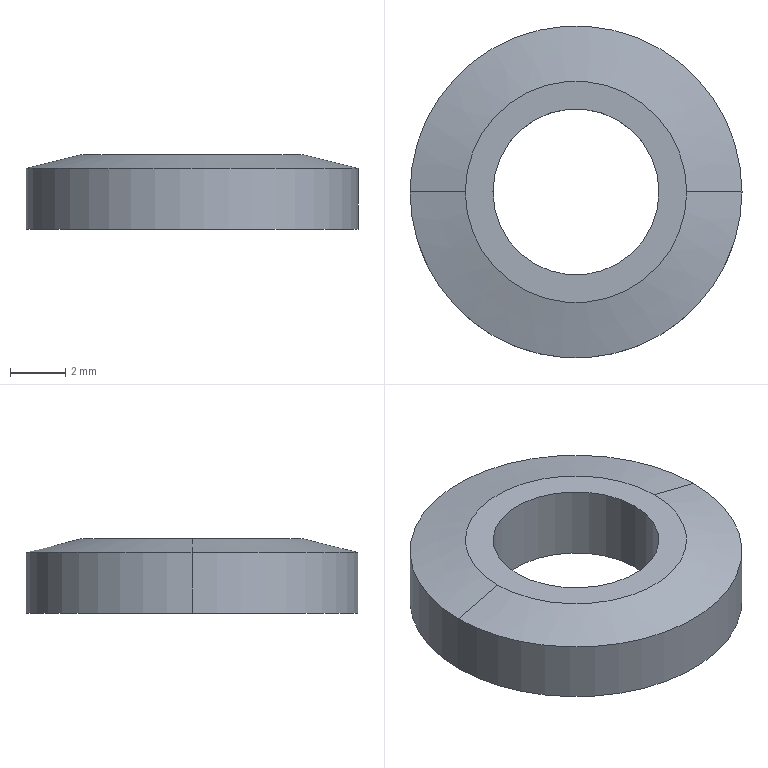Part | STEP file | 601-07-0094 | 1 solid | 8 faces | box 12 x 12 x 2.7 mm | volume 212.267 mm3 | cylinder 4 | cone 2 | plane 2 | commonest cylinder face diameters 6 x2 12 x2
STEP:
#1=CARTESIAN_POINT('',(0.,0.,0.));
#2=DIRECTION('',(0.,0.,1.));
#3=DIRECTION('',(1.,0.,0.));
#4=AXIS2_PLACEMENT_3D('',#1,#2,#3);
#5=CARTESIAN_POINT('',(4.,0.,2.7));
#6=VERTEX_POINT('',#5);
#7=CARTESIAN_POINT('',(-4.,0.,2.7));
#8=VERTEX_POINT('',#7);
#9=CARTESIAN_POINT('',(0.,0.,2.7));
#10=DIRECTION('',(0.,0.,1.));
#11=DIRECTION('',(1.,0.,0.));
#12=AXIS2_PLACEMENT_3D('',#9,#10,#11);
#13=CIRCLE('',#12,4.);
#14=CARTESIAN_POINT('',(0.,0.,2.7));
#15=DIRECTION('',(0.,0.,-1.));
#16=DIRECTION('',(-1.,0.,0.));
#17=AXIS2_PLACEMENT_3D('',#14,#15,#16);
#18=CONICAL_SURFACE('',#17,4.,1.326);
#19=CARTESIAN_POINT('',(3.142,0.));
#20=DIRECTION('',(-1.,0.));
#21=VECTOR('',#20,1.);
#22=LINE('',#19,#21);
#23=(GEOMETRIC_REPRESENTATION_CONTEXT(2)PARAMETRIC_REPRESENTATION_CONTEXT()REPRESENTATION_CONTEXT('',''));
#24=DEFINITIONAL_REPRESENTATION('',(#22),#23);
#25=PCURVE('',#18,#24);
#26=CARTESIAN_POINT('',(0.,0.,2.7));
#27=DIRECTION('',(0.,0.,1.));
#28=DIRECTION('',(1.,0.,0.));
#29=AXIS2_PLACEMENT_3D('',#26,#27,#28);
#30=PLANE('',#29);
#31=CARTESIAN_POINT('',(0.,0.));
#32=DIRECTION('',(1.,0.));
#33=AXIS2_PLACEMENT_2D('',#31,#32);
#34=CIRCLE('',#33,4.);
#35=(GEOMETRIC_REPRESENTATION_CONTEXT(2)PARAMETRIC_REPRESENTATION_CONTEXT()REPRESENTATION_CONTEXT('',''));
#36=DEFINITIONAL_REPRESENTATION('',(#34),#35);
#37=PCURVE('',#30,#36);
#38=SURFACE_CURVE('',#13,(#25,#37),.PCURVE_S1.);
#39=EDGE_CURVE('',#6,#8,#38,.T.);
#40=ORIENTED_EDGE('',*,*,#39,.F.);
#41=CARTESIAN_POINT('',(6.,0.,2.2));
#42=VERTEX_POINT('',#41);
#43=CARTESIAN_POINT('',(4.,0.,2.7));
#44=DIRECTION('',(0.9701,0.,-0.2425));
#45=VECTOR('',#44,1.);
#46=LINE('',#43,#45);
#47=CARTESIAN_POINT('',(3.142,0.));
#48=DIRECTION('',(0.,1.));
#49=VECTOR('',#48,1.);
#50=LINE('',#47,#49);
#51=(GEOMETRIC_REPRESENTATION_CONTEXT(2)PARAMETRIC_REPRESENTATION_CONTEXT()REPRESENTATION_CONTEXT('',''));
#52=DEFINITIONAL_REPRESENTATION('',(#50),#51);
#53=PCURVE('',#18,#52);
#54=CARTESIAN_POINT('',(0.,0.,2.7));
#55=DIRECTION('',(0.,0.,-1.));
#56=DIRECTION('',(-1.,0.,0.));
#57=AXIS2_PLACEMENT_3D('',#54,#55,#56);
#58=CONICAL_SURFACE('',#57,4.,1.326);
#59=CARTESIAN_POINT('',(3.142,0.));
#60=DIRECTION('',(0.,1.));
#61=VECTOR('',#60,1.);
#62=LINE('',#59,#61);
#63=(GEOMETRIC_REPRESENTATION_CONTEXT(2)PARAMETRIC_REPRESENTATION_CONTEXT()REPRESENTATION_CONTEXT('',''));
#64=DEFINITIONAL_REPRESENTATION('',(#62),#63);
#65=PCURVE('',#58,#64);
#66=SURFACE_CURVE('',#46,(#53,#65),.PCURVE_S1.);
#67=EDGE_CURVE('',#6,#42,#66,.T.);
#68=ORIENTED_EDGE('',*,*,#67,.T.);
#69=CARTESIAN_POINT('',(-6.,0.,2.2));
#70=VERTEX_POINT('',#69);
#71=CARTESIAN_POINT('',(0.,0.,2.2));
#72=DIRECTION('',(0.,0.,-1.));
#73=DIRECTION('',(1.,0.,0.));
#74=AXIS2_PLACEMENT_3D('',#71,#72,#73);
#75=CIRCLE('',#74,6.);
#76=CARTESIAN_POINT('',(-3.142,0.5));
#77=DIRECTION('',(1.,0.));
#78=VECTOR('',#77,1.);
#79=LINE('',#76,#78);
#80=(GEOMETRIC_REPRESENTATION_CONTEXT(2)PARAMETRIC_REPRESENTATION_CONTEXT()REPRESENTATION_CONTEXT('',''));
#81=DEFINITIONAL_REPRESENTATION('',(#79),#80);
#82=PCURVE('',#18,#81);
#83=CARTESIAN_POINT('',(0.,0.,2.7));
#84=DIRECTION('',(0.,0.,-1.));
#85=DIRECTION('',(-1.,0.,0.));
#86=AXIS2_PLACEMENT_3D('',#83,#84,#85);
#87=CYLINDRICAL_SURFACE('',#86,6.);
#88=CARTESIAN_POINT('',(-3.142,0.5));
#89=DIRECTION('',(1.,0.));
#90=VECTOR('',#89,1.);
#91=LINE('',#88,#90);
#92=(GEOMETRIC_REPRESENTATION_CONTEXT(2)PARAMETRIC_REPRESENTATION_CONTEXT()REPRESENTATION_CONTEXT('',''));
#93=DEFINITIONAL_REPRESENTATION('',(#91),#92);
#94=PCURVE('',#87,#93);
#95=SURFACE_CURVE('',#75,(#82,#94),.PCURVE_S1.);
#96=EDGE_CURVE('',#70,#42,#95,.T.);
#97=ORIENTED_EDGE('',*,*,#96,.F.);
#98=CARTESIAN_POINT('',(-4.,0.,2.7));
#99=DIRECTION('',(-0.9701,0.,-0.2425));
#100=VECTOR('',#99,1.);
#101=LINE('',#98,#100);
#102=CARTESIAN_POINT('',(0.,0.));
#103=DIRECTION('',(0.,1.));
#104=VECTOR('',#103,1.);
#105=LINE('',#102,#104);
#106=(GEOMETRIC_REPRESENTATION_CONTEXT(2)PARAMETRIC_REPRESENTATION_CONTEXT()REPRESENTATION_CONTEXT('',''));
#107=DEFINITIONAL_REPRESENTATION('',(#105),#106);
#108=PCURVE('',#18,#107);
#109=CARTESIAN_POINT('',(6.283,0.));
#110=DIRECTION('',(0.,1.));
#111=VECTOR('',#110,1.);
#112=LINE('',#109,#111);
#113=(GEOMETRIC_REPRESENTATION_CONTEXT(2)PARAMETRIC_REPRESENTATION_CONTEXT()REPRESENTATION_CONTEXT('',''));
#114=DEFINITIONAL_REPRESENTATION('',(#112),#113);
#115=PCURVE('',#58,#114);
#116=SURFACE_CURVE('',#101,(#108,#115),.PCURVE_S1.);
#117=EDGE_CURVE('',#8,#70,#116,.T.);
#118=ORIENTED_EDGE('',*,*,#117,.F.);
#119=EDGE_LOOP('',(#40,#68,#97,#118));
#120=FACE_BOUND('',#119,.T.);
#121=ADVANCED_FACE('',(#120),#18,.T.);
#122=CARTESIAN_POINT('',(3.,0.,0.));
#123=VERTEX_POINT('',#122);
#124=CARTESIAN_POINT('',(3.,0.,2.7));
#125=VERTEX_POINT('',#124);
#126=CARTESIAN_POINT('',(3.,0.,0.));
#127=DIRECTION('',(0.,0.,1.));
#128=VECTOR('',#127,1.);
#129=LINE('',#126,#128);
#130=CARTESIAN_POINT('',(0.,0.,0.));
#131=DIRECTION('',(0.,0.,1.));
#132=DIRECTION('',(1.,0.,0.));
#133=AXIS2_PLACEMENT_3D('',#130,#131,#132);
#134=CYLINDRICAL_SURFACE('',#133,3.);
#135=CARTESIAN_POINT('',(6.283,0.));
#136=DIRECTION('',(0.,1.));
#137=VECTOR('',#136,1.);
#138=LINE('',#135,#137);
#139=(GEOMETRIC_REPRESENTATION_CONTEXT(2)PARAMETRIC_REPRESENTATION_CONTEXT()REPRESENTATION_CONTEXT('',''));
#140=DEFINITIONAL_REPRESENTATION('',(#138),#139);
#141=PCURVE('',#134,#140);
#142=CARTESIAN_POINT('',(0.,0.,0.));
#143=DIRECTION('',(0.,0.,1.));
#144=DIRECTION('',(1.,0.,0.));
#145=AXIS2_PLACEMENT_3D('',#142,#143,#144);
#146=CYLINDRICAL_SURFACE('',#145,3.);
#147=CARTESIAN_POINT('',(0.,0.));
#148=DIRECTION('',(0.,1.));
#149=VECTOR('',#148,1.);
#150=LINE('',#147,#149);
#151=(GEOMETRIC_REPRESENTATION_CONTEXT(2)PARAMETRIC_REPRESENTATION_CONTEXT()REPRESENTATION_CONTEXT('',''));
#152=DEFINITIONAL_REPRESENTATION('',(#150),#151);
#153=PCURVE('',#146,#152);
#154=SURFACE_CURVE('',#129,(#141,#153),.PCURVE_S1.);
#155=EDGE_CURVE('',#123,#125,#154,.T.);
#156=ORIENTED_EDGE('',*,*,#155,.T.);
#157=CARTESIAN_POINT('',(-3.,0.,2.7));
#158=VERTEX_POINT('',#157);
#159=CARTESIAN_POINT('',(0.,0.,2.7));
#160=DIRECTION('',(0.,0.,1.));
#161=DIRECTION('',(1.,0.,0.));
#162=AXIS2_PLACEMENT_3D('',#159,#160,#161);
#163=CIRCLE('',#162,3.);
#164=CARTESIAN_POINT('',(0.,2.7));
#165=DIRECTION('',(1.,0.));
#166=VECTOR('',#165,1.);
#167=LINE('',#164,#166);
#168=(GEOMETRIC_REPRESENTATION_CONTEXT(2)PARAMETRIC_REPRESENTATION_CONTEXT()REPRESENTATION_CONTEXT('',''));
#169=DEFINITIONAL_REPRESENTATION('',(#167),#168);
#170=PCURVE('',#134,#169);
#171=CARTESIAN_POINT('',(0.,0.));
#172=DIRECTION('',(1.,0.));
#173=AXIS2_PLACEMENT_2D('',#171,#172);
#174=CIRCLE('',#173,3.);
#175=(GEOMETRIC_REPRESENTATION_CONTEXT(2)PARAMETRIC_REPRESENTATION_CONTEXT()REPRESENTATION_CONTEXT('',''));
#176=DEFINITIONAL_REPRESENTATION('',(#174),#175);
#177=PCURVE('',#30,#176);
#178=SURFACE_CURVE('',#163,(#170,#177),.PCURVE_S1.);
#179=EDGE_CURVE('',#158,#125,#178,.T.);
#180=ORIENTED_EDGE('',*,*,#179,.F.);
#181=CARTESIAN_POINT('',(-3.,0.,0.));
#182=VERTEX_POINT('',#181);
#183=CARTESIAN_POINT('',(-3.,0.,0.));
#184=DIRECTION('',(0.,0.,1.));
#185=VECTOR('',#184,1.);
#186=LINE('',#183,#185);
#187=CARTESIAN_POINT('',(3.142,0.));
#188=DIRECTION('',(0.,1.));
#189=VECTOR('',#188,1.);
#190=LINE('',#187,#189);
#191=(GEOMETRIC_REPRESENTATION_CONTEXT(2)PARAMETRIC_REPRESENTATION_CONTEXT()REPRESENTATION_CONTEXT('',''));
#192=DEFINITIONAL_REPRESENTATION('',(#190),#191);
#193=PCURVE('',#134,#192);
#194=CARTESIAN_POINT('',(3.142,0.));
#195=DIRECTION('',(0.,1.));
#196=VECTOR('',#195,1.);
#197=LINE('',#194,#196);
#198=(GEOMETRIC_REPRESENTATION_CONTEXT(2)PARAMETRIC_REPRESENTATION_CONTEXT()REPRESENTATION_CONTEXT('',''));
#199=DEFINITIONAL_REPRESENTATION('',(#197),#198);
#200=PCURVE('',#146,#199);
#201=SURFACE_CURVE('',#186,(#193,#200),.PCURVE_S1.);
#202=EDGE_CURVE('',#182,#158,#201,.T.);
#203=ORIENTED_EDGE('',*,*,#202,.F.);
#204=CARTESIAN_POINT('',(0.,0.,0.));
#205=DIRECTION('',(0.,0.,1.));
#206=DIRECTION('',(1.,0.,0.));
#207=AXIS2_PLACEMENT_3D('',#204,#205,#206);
#208=CIRCLE('',#207,3.);
#209=CARTESIAN_POINT('',(0.,0.));
#210=DIRECTION('',(1.,0.));
#211=VECTOR('',#210,1.);
#212=LINE('',#209,#211);
#213=(GEOMETRIC_REPRESENTATION_CONTEXT(2)PARAMETRIC_REPRESENTATION_CONTEXT()REPRESENTATION_CONTEXT('',''));
#214=DEFINITIONAL_REPRESENTATION('',(#212),#213);
#215=PCURVE('',#134,#214);
#216=CARTESIAN_POINT('',(0.,0.,0.));
#217=DIRECTION('',(0.,0.,1.));
#218=DIRECTION('',(1.,0.,0.));
#219=AXIS2_PLACEMENT_3D('',#216,#217,#218);
#220=PLANE('',#219);
#221=CARTESIAN_POINT('',(0.,0.));
#222=DIRECTION('',(1.,0.));
#223=AXIS2_PLACEMENT_2D('',#221,#222);
#224=CIRCLE('',#223,3.);
#225=(GEOMETRIC_REPRESENTATION_CONTEXT(2)PARAMETRIC_REPRESENTATION_CONTEXT()REPRESENTATION_CONTEXT('',''));
#226=DEFINITIONAL_REPRESENTATION('',(#224),#225);
#227=PCURVE('',#220,#226);
#228=SURFACE_CURVE('',#208,(#215,#227),.PCURVE_S1.);
#229=EDGE_CURVE('',#182,#123,#228,.T.);
#230=ORIENTED_EDGE('',*,*,#229,.T.);
#231=EDGE_LOOP('',(#156,#180,#203,#230));
#232=FACE_BOUND('',#231,.F.);
#233=ADVANCED_FACE('',(#232),#134,.F.);
#234=ORIENTED_EDGE('',*,*,#96,.T.);
#235=CARTESIAN_POINT('',(6.,0.,0.));
#236=VERTEX_POINT('',#235);
#237=CARTESIAN_POINT('',(6.,0.,2.7));
#238=DIRECTION('',(0.,0.,-1.));
#239=VECTOR('',#238,1.);
#240=LINE('',#237,#239);
#241=CARTESIAN_POINT('',(3.142,0.));
#242=DIRECTION('',(0.,1.));
#243=VECTOR('',#242,1.);
#244=LINE('',#241,#243);
#245=(GEOMETRIC_REPRESENTATION_CONTEXT(2)PARAMETRIC_REPRESENTATION_CONTEXT()REPRESENTATION_CONTEXT('',''));
#246=DEFINITIONAL_REPRESENTATION('',(#244),#245);
#247=PCURVE('',#87,#246);
#248=CARTESIAN_POINT('',(0.,0.,2.7));
#249=DIRECTION('',(0.,0.,-1.));
#250=DIRECTION('',(-1.,0.,0.));
#251=AXIS2_PLACEMENT_3D('',#248,#249,#250);
#252=CYLINDRICAL_SURFACE('',#251,6.);
#253=CARTESIAN_POINT('',(3.142,0.));
#254=DIRECTION('',(0.,1.));
#255=VECTOR('',#254,1.);
#256=LINE('',#253,#255);
#257=(GEOMETRIC_REPRESENTATION_CONTEXT(2)PARAMETRIC_REPRESENTATION_CONTEXT()REPRESENTATION_CONTEXT('',''));
#258=DEFINITIONAL_REPRESENTATION('',(#256),#257);
#259=PCURVE('',#252,#258);
#260=SURFACE_CURVE('',#240,(#247,#259),.PCURVE_S1.);
#261=EDGE_CURVE('',#42,#236,#260,.T.);
#262=ORIENTED_EDGE('',*,*,#261,.T.);
#263=CARTESIAN_POINT('',(-6.,0.,0.));
#264=VERTEX_POINT('',#263);
#265=CARTESIAN_POINT('',(0.,0.,0.));
#266=DIRECTION('',(0.,0.,1.));
#267=DIRECTION('',(1.,0.,0.));
#268=AXIS2_PLACEMENT_3D('',#265,#266,#267);
#269=CIRCLE('',#268,6.);
#270=CARTESIAN_POINT('',(3.142,2.7));
#271=DIRECTION('',(-1.,0.));
#272=VECTOR('',#271,1.);
#273=LINE('',#270,#272);
#274=(GEOMETRIC_REPRESENTATION_CONTEXT(2)PARAMETRIC_REPRESENTATION_CONTEXT()REPRESENTATION_CONTEXT('',''));
#275=DEFINITIONAL_REPRESENTATION('',(#273),#274);
#276=PCURVE('',#87,#275);
#277=CARTESIAN_POINT('',(0.,0.));
#278=DIRECTION('',(1.,0.));
#279=AXIS2_PLACEMENT_2D('',#277,#278);
#280=CIRCLE('',#279,6.);
#281=(GEOMETRIC_REPRESENTATION_CONTEXT(2)PARAMETRIC_REPRESENTATION_CONTEXT()REPRESENTATION_CONTEXT('',''));
#282=DEFINITIONAL_REPRESENTATION('',(#280),#281);
#283=PCURVE('',#220,#282);
#284=SURFACE_CURVE('',#269,(#276,#283),.PCURVE_S1.);
#285=EDGE_CURVE('',#236,#264,#284,.T.);
#286=ORIENTED_EDGE('',*,*,#285,.T.);
#287=CARTESIAN_POINT('',(-6.,0.,2.7));
#288=DIRECTION('',(0.,0.,-1.));
#289=VECTOR('',#288,1.);
#290=LINE('',#287,#289);
#291=CARTESIAN_POINT('',(0.,0.));
#292=DIRECTION('',(0.,1.));
#293=VECTOR('',#292,1.);
#294=LINE('',#291,#293);
#295=(GEOMETRIC_REPRESENTATION_CONTEXT(2)PARAMETRIC_REPRESENTATION_CONTEXT()REPRESENTATION_CONTEXT('',''));
#296=DEFINITIONAL_REPRESENTATION('',(#294),#295);
#297=PCURVE('',#87,#296);
#298=CARTESIAN_POINT('',(6.283,0.));
#299=DIRECTION('',(0.,1.));
#300=VECTOR('',#299,1.);
#301=LINE('',#298,#300);
#302=(GEOMETRIC_REPRESENTATION_CONTEXT(2)PARAMETRIC_REPRESENTATION_CONTEXT()REPRESENTATION_CONTEXT('',''));
#303=DEFINITIONAL_REPRESENTATION('',(#301),#302);
#304=PCURVE('',#252,#303);
#305=SURFACE_CURVE('',#290,(#297,#304),.PCURVE_S1.);
#306=EDGE_CURVE('',#70,#264,#305,.T.);
#307=ORIENTED_EDGE('',*,*,#306,.F.);
#308=EDGE_LOOP('',(#234,#262,#286,#307));
#309=FACE_BOUND('',#308,.T.);
#310=ADVANCED_FACE('',(#309),#87,.T.);
#311=ORIENTED_EDGE('',*,*,#261,.F.);
#312=CARTESIAN_POINT('',(0.,0.,2.2));
#313=DIRECTION('',(0.,0.,-1.));
#314=DIRECTION('',(1.,0.,0.));
#315=AXIS2_PLACEMENT_3D('',#312,#313,#314);
#316=CIRCLE('',#315,6.);
#317=CARTESIAN_POINT('',(3.142,0.5));
#318=DIRECTION('',(1.,0.));
#319=VECTOR('',#318,1.);
#320=LINE('',#317,#319);
#321=(GEOMETRIC_REPRESENTATION_CONTEXT(2)PARAMETRIC_REPRESENTATION_CONTEXT()REPRESENTATION_CONTEXT('',''));
#322=DEFINITIONAL_REPRESENTATION('',(#320),#321);
#323=PCURVE('',#252,#322);
#324=CARTESIAN_POINT('',(3.142,0.5));
#325=DIRECTION('',(1.,0.));
#326=VECTOR('',#325,1.);
#327=LINE('',#324,#326);
#328=(GEOMETRIC_REPRESENTATION_CONTEXT(2)PARAMETRIC_REPRESENTATION_CONTEXT()REPRESENTATION_CONTEXT('',''));
#329=DEFINITIONAL_REPRESENTATION('',(#327),#328);
#330=PCURVE('',#58,#329);
#331=SURFACE_CURVE('',#316,(#323,#330),.PCURVE_S1.);
#332=EDGE_CURVE('',#42,#70,#331,.T.);
#333=ORIENTED_EDGE('',*,*,#332,.T.);
#334=ORIENTED_EDGE('',*,*,#306,.T.);
#335=CARTESIAN_POINT('',(0.,0.,0.));
#336=DIRECTION('',(0.,0.,1.));
#337=DIRECTION('',(1.,0.,0.));
#338=AXIS2_PLACEMENT_3D('',#335,#336,#337);
#339=CIRCLE('',#338,6.);
#340=CARTESIAN_POINT('',(9.425,2.7));
#341=DIRECTION('',(-1.,0.));
#342=VECTOR('',#341,1.);
#343=LINE('',#340,#342);
#344=(GEOMETRIC_REPRESENTATION_CONTEXT(2)PARAMETRIC_REPRESENTATION_CONTEXT()REPRESENTATION_CONTEXT('',''));
#345=DEFINITIONAL_REPRESENTATION('',(#343),#344);
#346=PCURVE('',#252,#345);
#347=CARTESIAN_POINT('',(0.,0.));
#348=DIRECTION('',(1.,0.));
#349=AXIS2_PLACEMENT_2D('',#347,#348);
#350=CIRCLE('',#349,6.);
#351=(GEOMETRIC_REPRESENTATION_CONTEXT(2)PARAMETRIC_REPRESENTATION_CONTEXT()REPRESENTATION_CONTEXT('',''));
#352=DEFINITIONAL_REPRESENTATION('',(#350),#351);
#353=PCURVE('',#220,#352);
#354=SURFACE_CURVE('',#339,(#346,#353),.PCURVE_S1.);
#355=EDGE_CURVE('',#264,#236,#354,.T.);
#356=ORIENTED_EDGE('',*,*,#355,.T.);
#357=EDGE_LOOP('',(#311,#333,#334,#356));
#358=FACE_BOUND('',#357,.T.);
#359=ADVANCED_FACE('',(#358),#252,.T.);
#360=CARTESIAN_POINT('',(0.,0.,2.7));
#361=DIRECTION('',(0.,0.,1.));
#362=DIRECTION('',(1.,0.,0.));
#363=AXIS2_PLACEMENT_3D('',#360,#361,#362);
#364=CIRCLE('',#363,4.);
#365=CARTESIAN_POINT('',(0.,0.));
#366=DIRECTION('',(1.,0.));
#367=AXIS2_PLACEMENT_2D('',#365,#366);
#368=CIRCLE('',#367,4.);
#369=(GEOMETRIC_REPRESENTATION_CONTEXT(2)PARAMETRIC_REPRESENTATION_CONTEXT()REPRESENTATION_CONTEXT('',''));
#370=DEFINITIONAL_REPRESENTATION('',(#368),#369);
#371=PCURVE('',#30,#370);
#372=CARTESIAN_POINT('',(9.425,0.));
#373=DIRECTION('',(-1.,0.));
#374=VECTOR('',#373,1.);
#375=LINE('',#372,#374);
#376=(GEOMETRIC_REPRESENTATION_CONTEXT(2)PARAMETRIC_REPRESENTATION_CONTEXT()REPRESENTATION_CONTEXT('',''));
#377=DEFINITIONAL_REPRESENTATION('',(#375),#376);
#378=PCURVE('',#58,#377);
#379=SURFACE_CURVE('',#364,(#371,#378),.PCURVE_S1.);
#380=EDGE_CURVE('',#8,#6,#379,.T.);
#381=ORIENTED_EDGE('',*,*,#380,.T.);
#382=ORIENTED_EDGE('',*,*,#39,.T.);
#383=EDGE_LOOP('',(#381,#382));
#384=FACE_BOUND('',#383,.T.);
#385=CARTESIAN_POINT('',(0.,0.,2.7));
#386=DIRECTION('',(0.,0.,1.));
#387=DIRECTION('',(1.,0.,0.));
#388=AXIS2_PLACEMENT_3D('',#385,#386,#387);
#389=CIRCLE('',#388,3.);
#390=CARTESIAN_POINT('',(0.,0.));
#391=DIRECTION('',(1.,0.));
#392=AXIS2_PLACEMENT_2D('',#390,#391);
#393=CIRCLE('',#392,3.);
#394=(GEOMETRIC_REPRESENTATION_CONTEXT(2)PARAMETRIC_REPRESENTATION_CONTEXT()REPRESENTATION_CONTEXT('',''));
#395=DEFINITIONAL_REPRESENTATION('',(#393),#394);
#396=PCURVE('',#30,#395);
#397=CARTESIAN_POINT('',(0.,2.7));
#398=DIRECTION('',(1.,0.));
#399=VECTOR('',#398,1.);
#400=LINE('',#397,#399);
#401=(GEOMETRIC_REPRESENTATION_CONTEXT(2)PARAMETRIC_REPRESENTATION_CONTEXT()REPRESENTATION_CONTEXT('',''));
#402=DEFINITIONAL_REPRESENTATION('',(#400),#401);
#403=PCURVE('',#146,#402);
#404=SURFACE_CURVE('',#389,(#396,#403),.PCURVE_S1.);
#405=EDGE_CURVE('',#125,#158,#404,.T.);
#406=ORIENTED_EDGE('',*,*,#405,.F.);
#407=ORIENTED_EDGE('',*,*,#179,.F.);
#408=EDGE_LOOP('',(#406,#407));
#409=FACE_BOUND('',#408,.T.);
#410=ADVANCED_FACE('',(#384,#409),#30,.T.);
#411=CARTESIAN_POINT('',(0.,0.,0.));
#412=DIRECTION('',(0.,0.,1.));
#413=DIRECTION('',(1.,0.,0.));
#414=AXIS2_PLACEMENT_3D('',#411,#412,#413);
#415=CIRCLE('',#414,3.);
#416=CARTESIAN_POINT('',(0.,0.));
#417=DIRECTION('',(1.,0.));
#418=AXIS2_PLACEMENT_2D('',#416,#417);
#419=CIRCLE('',#418,3.);
#420=(GEOMETRIC_REPRESENTATION_CONTEXT(2)PARAMETRIC_REPRESENTATION_CONTEXT()REPRESENTATION_CONTEXT('',''));
#421=DEFINITIONAL_REPRESENTATION('',(#419),#420);
#422=PCURVE('',#220,#421);
#423=CARTESIAN_POINT('',(0.,0.));
#424=DIRECTION('',(1.,0.));
#425=VECTOR('',#424,1.);
#426=LINE('',#423,#425);
#427=(GEOMETRIC_REPRESENTATION_CONTEXT(2)PARAMETRIC_REPRESENTATION_CONTEXT()REPRESENTATION_CONTEXT('',''));
#428=DEFINITIONAL_REPRESENTATION('',(#426),#427);
#429=PCURVE('',#146,#428);
#430=SURFACE_CURVE('',#415,(#422,#429),.PCURVE_S1.);
#431=EDGE_CURVE('',#123,#182,#430,.T.);
#432=ORIENTED_EDGE('',*,*,#431,.T.);
#433=ORIENTED_EDGE('',*,*,#229,.T.);
#434=EDGE_LOOP('',(#432,#433));
#435=FACE_BOUND('',#434,.T.);
#436=ORIENTED_EDGE('',*,*,#355,.F.);
#437=ORIENTED_EDGE('',*,*,#285,.F.);
#438=EDGE_LOOP('',(#436,#437));
#439=FACE_BOUND('',#438,.T.);
#440=ADVANCED_FACE('',(#435,#439),#220,.F.);
#441=ORIENTED_EDGE('',*,*,#405,.F.);
#442=ORIENTED_EDGE('',*,*,#155,.F.);
#443=ORIENTED_EDGE('',*,*,#431,.T.);
#444=ORIENTED_EDGE('',*,*,#202,.T.);
#445=EDGE_LOOP('',(#441,#442,#443,#444));
#446=FACE_BOUND('',#445,.F.);
#447=ADVANCED_FACE('',(#446),#146,.F.);
#448=ORIENTED_EDGE('',*,*,#67,.F.);
#449=ORIENTED_EDGE('',*,*,#380,.F.);
#450=ORIENTED_EDGE('',*,*,#117,.T.);
#451=ORIENTED_EDGE('',*,*,#332,.F.);
#452=EDGE_LOOP('',(#448,#449,#450,#451));
#453=FACE_BOUND('',#452,.T.);
#454=ADVANCED_FACE('',(#453),#58,.T.);
#455=CLOSED_SHELL('',(#121,#233,#310,#359,#410,#440,#447,#454));
#456=MANIFOLD_SOLID_BREP('',#455);
#457=(LENGTH_UNIT()NAMED_UNIT(*)SI_UNIT(.MILLI.,.METRE.));
#458=UNCERTAINTY_MEASURE_WITH_UNIT(LENGTH_MEASURE(0.0000001),#457,'','');
#459=(NAMED_UNIT(*)PLANE_ANGLE_UNIT()SI_UNIT($,.RADIAN.));
#460=(NAMED_UNIT(*)SI_UNIT($,.STERADIAN.)SOLID_ANGLE_UNIT());
#461=(GEOMETRIC_REPRESENTATION_CONTEXT(3)GLOBAL_UNCERTAINTY_ASSIGNED_CONTEXT((#458))GLOBAL_UNIT_ASSIGNED_CONTEXT((#457,#459,#460))REPRESENTATION_CONTEXT('',''));
#462=ADVANCED_BREP_SHAPE_REPRESENTATION('',(#4,#456),#461);